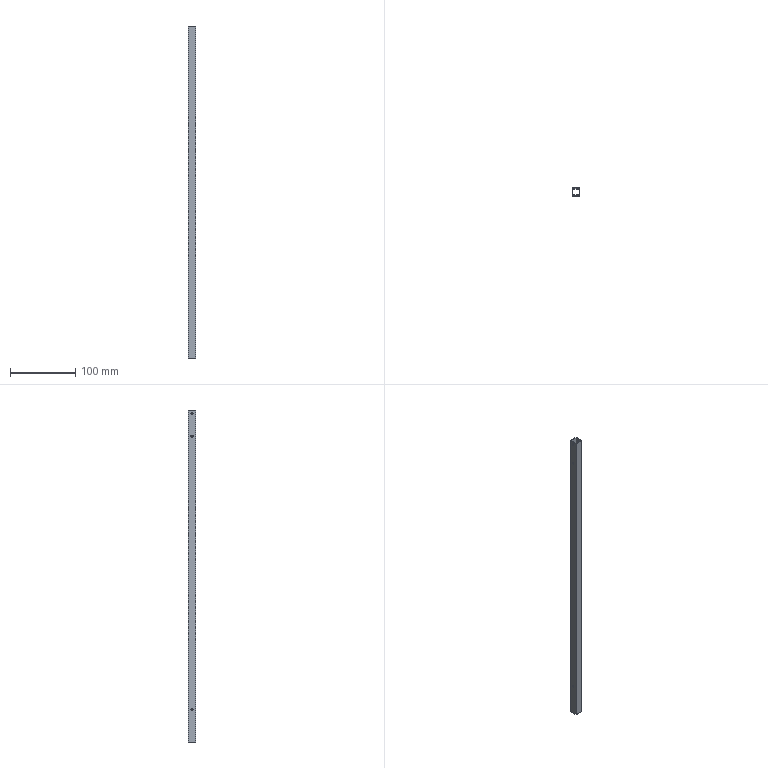Part | SolidWorks | features ICE 2, Extrusion 1 | 1 solid | 22 faces | box 12 x 12 x 508 mm | volume 22307 mm3 | cylinder 12 | plane 10 | commonest cylinder face diameters 3.1 x12
STEP:
#1=CARTESIAN_POINT('',(6.,0.,48.45));
#2=VERTEX_POINT('',#1);
#3=CARTESIAN_POINT('',(6.,0.,51.55));
#4=VERTEX_POINT('',#3);
#5=CARTESIAN_POINT('',(6.,0.,50.));
#6=DIRECTION('',(-1.,0.,0.));
#7=DIRECTION('',(0.,0.,1.));
#8=AXIS2_PLACEMENT_3D('',#5,#6,#7);
#9=CIRCLE('',#8,1.55);
#10=EDGE_CURVE('',#2,#4,#9,.T.);
#11=ORIENTED_EDGE('',*,*,#10,.F.);
#12=CARTESIAN_POINT('',(5.,0.,48.45));
#13=VERTEX_POINT('',#12);
#14=CARTESIAN_POINT('',(6.,0.,48.45));
#15=DIRECTION('',(-1.,0.,0.));
#16=VECTOR('',#15,1000.);
#17=LINE('',#14,#16);
#18=EDGE_CURVE('',#2,#13,#17,.T.);
#19=ORIENTED_EDGE('',*,*,#18,.T.);
#20=CARTESIAN_POINT('',(5.,0.,51.55));
#21=VERTEX_POINT('',#20);
#22=CARTESIAN_POINT('',(5.,0.,50.));
#23=DIRECTION('',(-1.,0.,0.));
#24=DIRECTION('',(0.,-1.,0.));
#25=AXIS2_PLACEMENT_3D('',#22,#23,#24);
#26=CIRCLE('',#25,1.55);
#27=EDGE_CURVE('',#13,#21,#26,.T.);
#28=ORIENTED_EDGE('',*,*,#27,.T.);
#29=CARTESIAN_POINT('',(6.,0.,51.55));
#30=DIRECTION('',(-1.,0.,0.));
#31=VECTOR('',#30,1000.);
#32=LINE('',#29,#31);
#33=EDGE_CURVE('',#4,#21,#32,.T.);
#34=ORIENTED_EDGE('',*,*,#33,.F.);
#35=EDGE_LOOP('',(#11,#19,#28,#34));
#36=FACE_OUTER_BOUND('',#35,.T.);
#37=CARTESIAN_POINT('',(6.,0.,50.));
#38=DIRECTION('',(-1.,0.,0.));
#39=DIRECTION('',(0.,0.,1.));
#40=AXIS2_PLACEMENT_3D('',#37,#38,#39);
#41=CYLINDRICAL_SURFACE('',#40,1.55);
#42=ADVANCED_FACE('',(#36),#41,.F.);
#43=CARTESIAN_POINT('',(6.,0.,466.583));
#44=VERTEX_POINT('',#43);
#45=CARTESIAN_POINT('',(6.,0.,469.683));
#46=VERTEX_POINT('',#45);
#47=CARTESIAN_POINT('',(6.,0.,468.133));
#48=DIRECTION('',(-1.,0.,0.));
#49=DIRECTION('',(0.,0.,1.));
#50=AXIS2_PLACEMENT_3D('',#47,#48,#49);
#51=CIRCLE('',#50,1.55);
#52=EDGE_CURVE('',#44,#46,#51,.T.);
#53=ORIENTED_EDGE('',*,*,#52,.F.);
#54=CARTESIAN_POINT('',(5.,0.,466.583));
#55=VERTEX_POINT('',#54);
#56=CARTESIAN_POINT('',(6.,0.,466.583));
#57=DIRECTION('',(-1.,0.,0.));
#58=VECTOR('',#57,1000.);
#59=LINE('',#56,#58);
#60=EDGE_CURVE('',#44,#55,#59,.T.);
#61=ORIENTED_EDGE('',*,*,#60,.T.);
#62=CARTESIAN_POINT('',(5.,0.,469.683));
#63=VERTEX_POINT('',#62);
#64=CARTESIAN_POINT('',(5.,0.,468.133));
#65=DIRECTION('',(-1.,0.,0.));
#66=DIRECTION('',(0.,-1.,0.));
#67=AXIS2_PLACEMENT_3D('',#64,#65,#66);
#68=CIRCLE('',#67,1.55);
#69=EDGE_CURVE('',#55,#63,#68,.T.);
#70=ORIENTED_EDGE('',*,*,#69,.T.);
#71=CARTESIAN_POINT('',(6.,0.,469.683));
#72=DIRECTION('',(-1.,0.,0.));
#73=VECTOR('',#72,1000.);
#74=LINE('',#71,#73);
#75=EDGE_CURVE('',#46,#63,#74,.T.);
#76=ORIENTED_EDGE('',*,*,#75,.F.);
#77=EDGE_LOOP('',(#53,#61,#70,#76));
#78=FACE_OUTER_BOUND('',#77,.T.);
#79=CARTESIAN_POINT('',(6.,0.,468.133));
#80=DIRECTION('',(-1.,0.,0.));
#81=DIRECTION('',(0.,0.,1.));
#82=AXIS2_PLACEMENT_3D('',#79,#80,#81);
#83=CYLINDRICAL_SURFACE('',#82,1.55);
#84=ADVANCED_FACE('',(#78),#83,.F.);
#85=CARTESIAN_POINT('',(6.,0.,501.583));
#86=VERTEX_POINT('',#85);
#87=CARTESIAN_POINT('',(6.,0.,504.683));
#88=VERTEX_POINT('',#87);
#89=CARTESIAN_POINT('',(6.,0.,503.133));
#90=DIRECTION('',(-1.,0.,0.));
#91=DIRECTION('',(0.,0.,1.));
#92=AXIS2_PLACEMENT_3D('',#89,#90,#91);
#93=CIRCLE('',#92,1.55);
#94=EDGE_CURVE('',#86,#88,#93,.T.);
#95=ORIENTED_EDGE('',*,*,#94,.F.);
#96=CARTESIAN_POINT('',(5.,0.,501.583));
#97=VERTEX_POINT('',#96);
#98=CARTESIAN_POINT('',(6.,0.,501.583));
#99=DIRECTION('',(-1.,0.,0.));
#100=VECTOR('',#99,1000.);
#101=LINE('',#98,#100);
#102=EDGE_CURVE('',#86,#97,#101,.T.);
#103=ORIENTED_EDGE('',*,*,#102,.T.);
#104=CARTESIAN_POINT('',(5.,0.,504.683));
#105=VERTEX_POINT('',#104);
#106=CARTESIAN_POINT('',(5.,0.,503.133));
#107=DIRECTION('',(-1.,0.,0.));
#108=DIRECTION('',(0.,-1.,0.));
#109=AXIS2_PLACEMENT_3D('',#106,#107,#108);
#110=CIRCLE('',#109,1.55);
#111=EDGE_CURVE('',#97,#105,#110,.T.);
#112=ORIENTED_EDGE('',*,*,#111,.T.);
#113=CARTESIAN_POINT('',(6.,0.,504.683));
#114=DIRECTION('',(-1.,0.,0.));
#115=VECTOR('',#114,1000.);
#116=LINE('',#113,#115);
#117=EDGE_CURVE('',#88,#105,#116,.T.);
#118=ORIENTED_EDGE('',*,*,#117,.F.);
#119=EDGE_LOOP('',(#95,#103,#112,#118));
#120=FACE_OUTER_BOUND('',#119,.T.);
#121=CARTESIAN_POINT('',(6.,0.,503.133));
#122=DIRECTION('',(-1.,0.,0.));
#123=DIRECTION('',(0.,0.,1.));
#124=AXIS2_PLACEMENT_3D('',#121,#122,#123);
#125=CYLINDRICAL_SURFACE('',#124,1.55);
#126=ADVANCED_FACE('',(#120),#125,.F.);
#127=CARTESIAN_POINT('',(-5.,0.,51.55));
#128=VERTEX_POINT('',#127);
#129=CARTESIAN_POINT('',(-5.,0.,48.45));
#130=VERTEX_POINT('',#129);
#131=CARTESIAN_POINT('',(-5.,0.,50.));
#132=DIRECTION('',(1.,0.,0.));
#133=DIRECTION('',(0.,0.,-1.));
#134=AXIS2_PLACEMENT_3D('',#131,#132,#133);
#135=CIRCLE('',#134,1.55);
#136=EDGE_CURVE('',#128,#130,#135,.T.);
#137=ORIENTED_EDGE('',*,*,#136,.T.);
#138=CARTESIAN_POINT('',(-6.,0.,48.45));
#139=VERTEX_POINT('',#138);
#140=CARTESIAN_POINT('',(6.,0.,48.45));
#141=DIRECTION('',(-1.,0.,0.));
#142=VECTOR('',#141,1000.);
#143=LINE('',#140,#142);
#144=EDGE_CURVE('',#130,#139,#143,.T.);
#145=ORIENTED_EDGE('',*,*,#144,.T.);
#146=CARTESIAN_POINT('',(-6.,0.,51.55));
#147=VERTEX_POINT('',#146);
#148=CARTESIAN_POINT('',(-6.,0.,50.));
#149=DIRECTION('',(1.,0.,0.));
#150=DIRECTION('',(0.,0.,-1.));
#151=AXIS2_PLACEMENT_3D('',#148,#149,#150);
#152=CIRCLE('',#151,1.55);
#153=EDGE_CURVE('',#147,#139,#152,.T.);
#154=ORIENTED_EDGE('',*,*,#153,.F.);
#155=CARTESIAN_POINT('',(6.,0.,51.55));
#156=DIRECTION('',(-1.,0.,0.));
#157=VECTOR('',#156,1000.);
#158=LINE('',#155,#157);
#159=EDGE_CURVE('',#128,#147,#158,.T.);
#160=ORIENTED_EDGE('',*,*,#159,.F.);
#161=EDGE_LOOP('',(#137,#145,#154,#160));
#162=FACE_OUTER_BOUND('',#161,.T.);
#163=CARTESIAN_POINT('',(6.,0.,50.));
#164=DIRECTION('',(-1.,0.,0.));
#165=DIRECTION('',(0.,0.,1.));
#166=AXIS2_PLACEMENT_3D('',#163,#164,#165);
#167=CYLINDRICAL_SURFACE('',#166,1.55);
#168=ADVANCED_FACE('',(#162),#167,.F.);
#169=CARTESIAN_POINT('',(-5.,0.,469.683));
#170=VERTEX_POINT('',#169);
#171=CARTESIAN_POINT('',(-5.,0.,466.583));
#172=VERTEX_POINT('',#171);
#173=CARTESIAN_POINT('',(-5.,0.,468.133));
#174=DIRECTION('',(1.,0.,0.));
#175=DIRECTION('',(0.,0.,-1.));
#176=AXIS2_PLACEMENT_3D('',#173,#174,#175);
#177=CIRCLE('',#176,1.55);
#178=EDGE_CURVE('',#170,#172,#177,.T.);
#179=ORIENTED_EDGE('',*,*,#178,.T.);
#180=CARTESIAN_POINT('',(-6.,0.,466.583));
#181=VERTEX_POINT('',#180);
#182=CARTESIAN_POINT('',(6.,0.,466.583));
#183=DIRECTION('',(-1.,0.,0.));
#184=VECTOR('',#183,1000.);
#185=LINE('',#182,#184);
#186=EDGE_CURVE('',#172,#181,#185,.T.);
#187=ORIENTED_EDGE('',*,*,#186,.T.);
#188=CARTESIAN_POINT('',(-6.,0.,469.683));
#189=VERTEX_POINT('',#188);
#190=CARTESIAN_POINT('',(-6.,0.,468.133));
#191=DIRECTION('',(1.,0.,0.));
#192=DIRECTION('',(0.,0.,-1.));
#193=AXIS2_PLACEMENT_3D('',#190,#191,#192);
#194=CIRCLE('',#193,1.55);
#195=EDGE_CURVE('',#189,#181,#194,.T.);
#196=ORIENTED_EDGE('',*,*,#195,.F.);
#197=CARTESIAN_POINT('',(6.,0.,469.683));
#198=DIRECTION('',(-1.,0.,0.));
#199=VECTOR('',#198,1000.);
#200=LINE('',#197,#199);
#201=EDGE_CURVE('',#170,#189,#200,.T.);
#202=ORIENTED_EDGE('',*,*,#201,.F.);
#203=EDGE_LOOP('',(#179,#187,#196,#202));
#204=FACE_OUTER_BOUND('',#203,.T.);
#205=CARTESIAN_POINT('',(6.,0.,468.133));
#206=DIRECTION('',(-1.,0.,0.));
#207=DIRECTION('',(0.,0.,1.));
#208=AXIS2_PLACEMENT_3D('',#205,#206,#207);
#209=CYLINDRICAL_SURFACE('',#208,1.55);
#210=ADVANCED_FACE('',(#204),#209,.F.);
#211=CARTESIAN_POINT('',(-5.,0.,504.683));
#212=VERTEX_POINT('',#211);
#213=CARTESIAN_POINT('',(-5.,0.,501.583));
#214=VERTEX_POINT('',#213);
#215=CARTESIAN_POINT('',(-5.,0.,503.133));
#216=DIRECTION('',(1.,0.,0.));
#217=DIRECTION('',(0.,0.,-1.));
#218=AXIS2_PLACEMENT_3D('',#215,#216,#217);
#219=CIRCLE('',#218,1.55);
#220=EDGE_CURVE('',#212,#214,#219,.T.);
#221=ORIENTED_EDGE('',*,*,#220,.T.);
#222=CARTESIAN_POINT('',(-6.,0.,501.583));
#223=VERTEX_POINT('',#222);
#224=CARTESIAN_POINT('',(6.,0.,501.583));
#225=DIRECTION('',(-1.,0.,0.));
#226=VECTOR('',#225,1000.);
#227=LINE('',#224,#226);
#228=EDGE_CURVE('',#214,#223,#227,.T.);
#229=ORIENTED_EDGE('',*,*,#228,.T.);
#230=CARTESIAN_POINT('',(-6.,0.,504.683));
#231=VERTEX_POINT('',#230);
#232=CARTESIAN_POINT('',(-6.,0.,503.133));
#233=DIRECTION('',(1.,0.,0.));
#234=DIRECTION('',(0.,0.,-1.));
#235=AXIS2_PLACEMENT_3D('',#232,#233,#234);
#236=CIRCLE('',#235,1.55);
#237=EDGE_CURVE('',#231,#223,#236,.T.);
#238=ORIENTED_EDGE('',*,*,#237,.F.);
#239=CARTESIAN_POINT('',(6.,0.,504.683));
#240=DIRECTION('',(-1.,0.,0.));
#241=VECTOR('',#240,1000.);
#242=LINE('',#239,#241);
#243=EDGE_CURVE('',#212,#231,#242,.T.);
#244=ORIENTED_EDGE('',*,*,#243,.F.);
#245=EDGE_LOOP('',(#221,#229,#238,#244));
#246=FACE_OUTER_BOUND('',#245,.T.);
#247=CARTESIAN_POINT('',(6.,0.,503.133));
#248=DIRECTION('',(-1.,0.,0.));
#249=DIRECTION('',(0.,0.,1.));
#250=AXIS2_PLACEMENT_3D('',#247,#248,#249);
#251=CYLINDRICAL_SURFACE('',#250,1.55);
#252=ADVANCED_FACE('',(#246),#251,.F.);
#253=CARTESIAN_POINT('',(6.,0.,503.133));
#254=DIRECTION('',(-1.,0.,0.));
#255=DIRECTION('',(0.,0.,1.));
#256=AXIS2_PLACEMENT_3D('',#253,#254,#255);
#257=CIRCLE('',#256,1.55);
#258=EDGE_CURVE('',#88,#86,#257,.T.);
#259=ORIENTED_EDGE('',*,*,#258,.T.);
#260=ORIENTED_EDGE('',*,*,#94,.T.);
#261=EDGE_LOOP('',(#259,#260));
#262=FACE_BOUND('',#261,.T.);
#263=CARTESIAN_POINT('',(6.,0.,468.133));
#264=DIRECTION('',(-1.,0.,0.));
#265=DIRECTION('',(0.,0.,1.));
#266=AXIS2_PLACEMENT_3D('',#263,#264,#265);
#267=CIRCLE('',#266,1.55);
#268=EDGE_CURVE('',#46,#44,#267,.T.);
#269=ORIENTED_EDGE('',*,*,#268,.T.);
#270=ORIENTED_EDGE('',*,*,#52,.T.);
#271=EDGE_LOOP('',(#269,#270));
#272=FACE_BOUND('',#271,.T.);
#273=CARTESIAN_POINT('',(6.,0.,50.));
#274=DIRECTION('',(-1.,0.,0.));
#275=DIRECTION('',(0.,0.,1.));
#276=AXIS2_PLACEMENT_3D('',#273,#274,#275);
#277=CIRCLE('',#276,1.55);
#278=EDGE_CURVE('',#4,#2,#277,.T.);
#279=ORIENTED_EDGE('',*,*,#278,.T.);
#280=ORIENTED_EDGE('',*,*,#10,.T.);
#281=EDGE_LOOP('',(#279,#280));
#282=FACE_BOUND('',#281,.T.);
#283=CARTESIAN_POINT('',(6.,-6.,508.));
#284=VERTEX_POINT('',#283);
#285=CARTESIAN_POINT('',(6.,6.,508.));
#286=VERTEX_POINT('',#285);
#287=CARTESIAN_POINT('',(6.,-6.,508.));
#288=DIRECTION('',(0.,1.,0.));
#289=VECTOR('',#288,1000.);
#290=LINE('',#287,#289);
#291=EDGE_CURVE('',#284,#286,#290,.T.);
#292=ORIENTED_EDGE('',*,*,#291,.F.);
#293=CARTESIAN_POINT('',(6.,-6.,0.));
#294=VERTEX_POINT('',#293);
#295=CARTESIAN_POINT('',(6.,-6.,516.));
#296=DIRECTION('',(0.,0.,-1.));
#297=VECTOR('',#296,1000.);
#298=LINE('',#295,#297);
#299=EDGE_CURVE('',#284,#294,#298,.T.);
#300=ORIENTED_EDGE('',*,*,#299,.T.);
#301=CARTESIAN_POINT('',(6.,6.,0.));
#302=VERTEX_POINT('',#301);
#303=CARTESIAN_POINT('',(6.,-6.,0.));
#304=DIRECTION('',(0.,1.,0.));
#305=VECTOR('',#304,1000.);
#306=LINE('',#303,#305);
#307=EDGE_CURVE('',#294,#302,#306,.T.);
#308=ORIENTED_EDGE('',*,*,#307,.T.);
#309=CARTESIAN_POINT('',(6.,6.,516.));
#310=DIRECTION('',(0.,0.,-1.));
#311=VECTOR('',#310,1000.);
#312=LINE('',#309,#311);
#313=EDGE_CURVE('',#286,#302,#312,.T.);
#314=ORIENTED_EDGE('',*,*,#313,.F.);
#315=EDGE_LOOP('',(#292,#300,#308,#314));
#316=FACE_OUTER_BOUND('',#315,.T.);
#317=CARTESIAN_POINT('',(6.,-6.,516.));
#318=DIRECTION('',(-1.,0.,0.));
#319=DIRECTION('',(0.,0.,1.));
#320=AXIS2_PLACEMENT_3D('',#317,#318,#319);
#321=PLANE('',#320);
#322=ADVANCED_FACE('',(#262,#272,#282,#316),#321,.F.);
#323=CARTESIAN_POINT('',(-6.,6.,508.));
#324=VERTEX_POINT('',#323);
#325=CARTESIAN_POINT('',(6.,6.,508.));
#326=DIRECTION('',(-1.,0.,0.));
#327=VECTOR('',#326,1000.);
#328=LINE('',#325,#327);
#329=EDGE_CURVE('',#286,#324,#328,.T.);
#330=ORIENTED_EDGE('',*,*,#329,.F.);
#331=ORIENTED_EDGE('',*,*,#313,.T.);
#332=CARTESIAN_POINT('',(-6.,6.,0.));
#333=VERTEX_POINT('',#332);
#334=CARTESIAN_POINT('',(-6.,6.,0.));
#335=DIRECTION('',(-1.,0.,0.));
#336=VECTOR('',#335,1000.);
#337=LINE('',#334,#336);
#338=EDGE_CURVE('',#302,#333,#337,.T.);
#339=ORIENTED_EDGE('',*,*,#338,.T.);
#340=CARTESIAN_POINT('',(-6.,6.,516.));
#341=DIRECTION('',(0.,0.,-1.));
#342=VECTOR('',#341,1000.);
#343=LINE('',#340,#342);
#344=EDGE_CURVE('',#324,#333,#343,.T.);
#345=ORIENTED_EDGE('',*,*,#344,.F.);
#346=EDGE_LOOP('',(#330,#331,#339,#345));
#347=FACE_OUTER_BOUND('',#346,.T.);
#348=CARTESIAN_POINT('',(-6.,6.,516.));
#349=DIRECTION('',(0.,-1.,0.));
#350=DIRECTION('',(0.,0.,-1.));
#351=AXIS2_PLACEMENT_3D('',#348,#349,#350);
#352=PLANE('',#351);
#353=ADVANCED_FACE('',(#347),#352,.F.);
#354=ORIENTED_EDGE('',*,*,#237,.T.);
#355=CARTESIAN_POINT('',(-6.,0.,503.133));
#356=DIRECTION('',(1.,0.,0.));
#357=DIRECTION('',(0.,0.,-1.));
#358=AXIS2_PLACEMENT_3D('',#355,#356,#357);
#359=CIRCLE('',#358,1.55);
#360=EDGE_CURVE('',#223,#231,#359,.T.);
#361=ORIENTED_EDGE('',*,*,#360,.T.);
#362=EDGE_LOOP('',(#354,#361));
#363=FACE_BOUND('',#362,.T.);
#364=ORIENTED_EDGE('',*,*,#195,.T.);
#365=CARTESIAN_POINT('',(-6.,0.,468.133));
#366=DIRECTION('',(1.,0.,0.));
#367=DIRECTION('',(0.,0.,-1.));
#368=AXIS2_PLACEMENT_3D('',#365,#366,#367);
#369=CIRCLE('',#368,1.55);
#370=EDGE_CURVE('',#181,#189,#369,.T.);
#371=ORIENTED_EDGE('',*,*,#370,.T.);
#372=EDGE_LOOP('',(#364,#371));
#373=FACE_BOUND('',#372,.T.);
#374=ORIENTED_EDGE('',*,*,#153,.T.);
#375=CARTESIAN_POINT('',(-6.,0.,50.));
#376=DIRECTION('',(1.,0.,0.));
#377=DIRECTION('',(0.,0.,-1.));
#378=AXIS2_PLACEMENT_3D('',#375,#376,#377);
#379=CIRCLE('',#378,1.55);
#380=EDGE_CURVE('',#139,#147,#379,.T.);
#381=ORIENTED_EDGE('',*,*,#380,.T.);
#382=EDGE_LOOP('',(#374,#381));
#383=FACE_BOUND('',#382,.T.);
#384=CARTESIAN_POINT('',(-6.,-6.,508.));
#385=VERTEX_POINT('',#384);
#386=CARTESIAN_POINT('',(-6.,6.,508.));
#387=DIRECTION('',(0.,-1.,0.));
#388=VECTOR('',#387,1000.);
#389=LINE('',#386,#388);
#390=EDGE_CURVE('',#324,#385,#389,.T.);
#391=ORIENTED_EDGE('',*,*,#390,.F.);
#392=ORIENTED_EDGE('',*,*,#344,.T.);
#393=CARTESIAN_POINT('',(-6.,-6.,0.));
#394=VERTEX_POINT('',#393);
#395=CARTESIAN_POINT('',(-6.,-6.,0.));
#396=DIRECTION('',(0.,-1.,0.));
#397=VECTOR('',#396,1000.);
#398=LINE('',#395,#397);
#399=EDGE_CURVE('',#333,#394,#398,.T.);
#400=ORIENTED_EDGE('',*,*,#399,.T.);
#401=CARTESIAN_POINT('',(-6.,-6.,516.));
#402=DIRECTION('',(0.,0.,-1.));
#403=VECTOR('',#402,1000.);
#404=LINE('',#401,#403);
#405=EDGE_CURVE('',#385,#394,#404,.T.);
#406=ORIENTED_EDGE('',*,*,#405,.F.);
#407=EDGE_LOOP('',(#391,#392,#400,#406));
#408=FACE_OUTER_BOUND('',#407,.T.);
#409=CARTESIAN_POINT('',(-6.,-6.,516.));
#410=DIRECTION('',(1.,0.,0.));
#411=DIRECTION('',(0.,0.,-1.));
#412=AXIS2_PLACEMENT_3D('',#409,#410,#411);
#413=PLANE('',#412);
#414=ADVANCED_FACE('',(#363,#373,#383,#408),#413,.F.);
#415=CARTESIAN_POINT('',(-6.,-6.,508.));
#416=DIRECTION('',(1.,0.,0.));
#417=VECTOR('',#416,1000.);
#418=LINE('',#415,#417);
#419=EDGE_CURVE('',#385,#284,#418,.T.);
#420=ORIENTED_EDGE('',*,*,#419,.F.);
#421=ORIENTED_EDGE('',*,*,#405,.T.);
#422=CARTESIAN_POINT('',(-6.,-6.,0.));
#423=DIRECTION('',(1.,0.,0.));
#424=VECTOR('',#423,1000.);
#425=LINE('',#422,#424);
#426=EDGE_CURVE('',#394,#294,#425,.T.);
#427=ORIENTED_EDGE('',*,*,#426,.T.);
#428=ORIENTED_EDGE('',*,*,#299,.F.);
#429=EDGE_LOOP('',(#420,#421,#427,#428));
#430=FACE_OUTER_BOUND('',#429,.T.);
#431=CARTESIAN_POINT('',(-6.,-6.,516.));
#432=DIRECTION('',(0.,1.,0.));
#433=DIRECTION('',(0.,0.,1.));
#434=AXIS2_PLACEMENT_3D('',#431,#432,#433);
#435=PLANE('',#434);
#436=ADVANCED_FACE('',(#430),#435,.F.);
#437=CARTESIAN_POINT('',(-5.,-5.,508.));
#438=VERTEX_POINT('',#437);
#439=CARTESIAN_POINT('',(-5.,-5.,0.));
#440=VERTEX_POINT('',#439);
#441=CARTESIAN_POINT('',(-5.,-5.,516.));
#442=DIRECTION('',(0.,0.,-1.));
#443=VECTOR('',#442,1000.);
#444=LINE('',#441,#443);
#445=EDGE_CURVE('',#438,#440,#444,.T.);
#446=ORIENTED_EDGE('',*,*,#445,.F.);
#447=CARTESIAN_POINT('',(5.,-5.,508.));
#448=VERTEX_POINT('',#447);
#449=CARTESIAN_POINT('',(-5.,-5.,508.));
#450=DIRECTION('',(1.,0.,0.));
#451=VECTOR('',#450,1000.);
#452=LINE('',#449,#451);
#453=EDGE_CURVE('',#438,#448,#452,.T.);
#454=ORIENTED_EDGE('',*,*,#453,.T.);
#455=CARTESIAN_POINT('',(5.,-5.,0.));
#456=VERTEX_POINT('',#455);
#457=CARTESIAN_POINT('',(5.,-5.,516.));
#458=DIRECTION('',(0.,0.,-1.));
#459=VECTOR('',#458,1000.);
#460=LINE('',#457,#459);
#461=EDGE_CURVE('',#448,#456,#460,.T.);
#462=ORIENTED_EDGE('',*,*,#461,.T.);
#463=CARTESIAN_POINT('',(-5.,-5.,0.));
#464=DIRECTION('',(1.,0.,0.));
#465=VECTOR('',#464,1000.);
#466=LINE('',#463,#465);
#467=EDGE_CURVE('',#440,#456,#466,.T.);
#468=ORIENTED_EDGE('',*,*,#467,.F.);
#469=EDGE_LOOP('',(#446,#454,#462,#468));
#470=FACE_OUTER_BOUND('',#469,.T.);
#471=CARTESIAN_POINT('',(-5.,-5.,516.));
#472=DIRECTION('',(0.,1.,0.));
#473=DIRECTION('',(0.,0.,1.));
#474=AXIS2_PLACEMENT_3D('',#471,#472,#473);
#475=PLANE('',#474);
#476=ADVANCED_FACE('',(#470),#475,.T.);
#477=CARTESIAN_POINT('',(5.,0.,50.));
#478=DIRECTION('',(-1.,0.,0.));
#479=DIRECTION('',(0.,-1.,0.));
#480=AXIS2_PLACEMENT_3D('',#477,#478,#479);
#481=CIRCLE('',#480,1.55);
#482=EDGE_CURVE('',#21,#13,#481,.T.);
#483=ORIENTED_EDGE('',*,*,#482,.F.);
#484=ORIENTED_EDGE('',*,*,#27,.F.);
#485=EDGE_LOOP('',(#483,#484));
#486=FACE_BOUND('',#485,.T.);
#487=CARTESIAN_POINT('',(5.,0.,468.133));
#488=DIRECTION('',(-1.,0.,0.));
#489=DIRECTION('',(0.,-1.,0.));
#490=AXIS2_PLACEMENT_3D('',#487,#488,#489);
#491=CIRCLE('',#490,1.55);
#492=EDGE_CURVE('',#63,#55,#491,.T.);
#493=ORIENTED_EDGE('',*,*,#492,.F.);
#494=ORIENTED_EDGE('',*,*,#69,.F.);
#495=EDGE_LOOP('',(#493,#494));
#496=FACE_BOUND('',#495,.T.);
#497=CARTESIAN_POINT('',(5.,0.,503.133));
#498=DIRECTION('',(-1.,0.,0.));
#499=DIRECTION('',(0.,-1.,0.));
#500=AXIS2_PLACEMENT_3D('',#497,#498,#499);
#501=CIRCLE('',#500,1.55);
#502=EDGE_CURVE('',#105,#97,#501,.T.);
#503=ORIENTED_EDGE('',*,*,#502,.F.);
#504=ORIENTED_EDGE('',*,*,#111,.F.);
#505=EDGE_LOOP('',(#503,#504));
#506=FACE_BOUND('',#505,.T.);
#507=ORIENTED_EDGE('',*,*,#461,.F.);
#508=CARTESIAN_POINT('',(5.,5.,508.));
#509=VERTEX_POINT('',#508);
#510=CARTESIAN_POINT('',(5.,-5.,508.));
#511=DIRECTION('',(0.,1.,0.));
#512=VECTOR('',#511,1000.);
#513=LINE('',#510,#512);
#514=EDGE_CURVE('',#448,#509,#513,.T.);
#515=ORIENTED_EDGE('',*,*,#514,.T.);
#516=CARTESIAN_POINT('',(5.,5.,0.));
#517=VERTEX_POINT('',#516);
#518=CARTESIAN_POINT('',(5.,5.,516.));
#519=DIRECTION('',(0.,0.,-1.));
#520=VECTOR('',#519,1000.);
#521=LINE('',#518,#520);
#522=EDGE_CURVE('',#509,#517,#521,.T.);
#523=ORIENTED_EDGE('',*,*,#522,.T.);
#524=CARTESIAN_POINT('',(5.,-5.,0.));
#525=DIRECTION('',(0.,1.,0.));
#526=VECTOR('',#525,1000.);
#527=LINE('',#524,#526);
#528=EDGE_CURVE('',#456,#517,#527,.T.);
#529=ORIENTED_EDGE('',*,*,#528,.F.);
#530=EDGE_LOOP('',(#507,#515,#523,#529));
#531=FACE_OUTER_BOUND('',#530,.T.);
#532=CARTESIAN_POINT('',(5.,-5.,516.));
#533=DIRECTION('',(-1.,0.,0.));
#534=DIRECTION('',(0.,-1.,0.));
#535=AXIS2_PLACEMENT_3D('',#532,#533,#534);
#536=PLANE('',#535);
#537=ADVANCED_FACE('',(#486,#496,#506,#531),#536,.T.);
#538=ORIENTED_EDGE('',*,*,#522,.F.);
#539=CARTESIAN_POINT('',(-5.,5.,508.));
#540=VERTEX_POINT('',#539);
#541=CARTESIAN_POINT('',(5.,5.,508.));
#542=DIRECTION('',(-1.,0.,0.));
#543=VECTOR('',#542,1000.);
#544=LINE('',#541,#543);
#545=EDGE_CURVE('',#509,#540,#544,.T.);
#546=ORIENTED_EDGE('',*,*,#545,.T.);
#547=CARTESIAN_POINT('',(-5.,5.,0.));
#548=VERTEX_POINT('',#547);
#549=CARTESIAN_POINT('',(-5.,5.,516.));
#550=DIRECTION('',(0.,0.,-1.));
#551=VECTOR('',#550,1000.);
#552=LINE('',#549,#551);
#553=EDGE_CURVE('',#540,#548,#552,.T.);
#554=ORIENTED_EDGE('',*,*,#553,.T.);
#555=CARTESIAN_POINT('',(-5.,5.,0.));
#556=DIRECTION('',(-1.,0.,0.));
#557=VECTOR('',#556,1000.);
#558=LINE('',#555,#557);
#559=EDGE_CURVE('',#517,#548,#558,.T.);
#560=ORIENTED_EDGE('',*,*,#559,.F.);
#561=EDGE_LOOP('',(#538,#546,#554,#560));
#562=FACE_OUTER_BOUND('',#561,.T.);
#563=CARTESIAN_POINT('',(-5.,5.,516.));
#564=DIRECTION('',(0.,-1.,0.));
#565=DIRECTION('',(0.,0.,-1.));
#566=AXIS2_PLACEMENT_3D('',#563,#564,#565);
#567=PLANE('',#566);
#568=ADVANCED_FACE('',(#562),#567,.T.);
#569=ORIENTED_EDGE('',*,*,#136,.F.);
#570=CARTESIAN_POINT('',(-5.,0.,50.));
#571=DIRECTION('',(1.,0.,0.));
#572=DIRECTION('',(0.,0.,-1.));
#573=AXIS2_PLACEMENT_3D('',#570,#571,#572);
#574=CIRCLE('',#573,1.55);
#575=EDGE_CURVE('',#130,#128,#574,.T.);
#576=ORIENTED_EDGE('',*,*,#575,.F.);
#577=EDGE_LOOP('',(#569,#576));
#578=FACE_BOUND('',#577,.T.);
#579=ORIENTED_EDGE('',*,*,#178,.F.);
#580=CARTESIAN_POINT('',(-5.,0.,468.133));
#581=DIRECTION('',(1.,0.,0.));
#582=DIRECTION('',(0.,0.,-1.));
#583=AXIS2_PLACEMENT_3D('',#580,#581,#582);
#584=CIRCLE('',#583,1.55);
#585=EDGE_CURVE('',#172,#170,#584,.T.);
#586=ORIENTED_EDGE('',*,*,#585,.F.);
#587=EDGE_LOOP('',(#579,#586));
#588=FACE_BOUND('',#587,.T.);
#589=ORIENTED_EDGE('',*,*,#220,.F.);
#590=CARTESIAN_POINT('',(-5.,0.,503.133));
#591=DIRECTION('',(1.,0.,0.));
#592=DIRECTION('',(0.,0.,-1.));
#593=AXIS2_PLACEMENT_3D('',#590,#591,#592);
#594=CIRCLE('',#593,1.55);
#595=EDGE_CURVE('',#214,#212,#594,.T.);
#596=ORIENTED_EDGE('',*,*,#595,.F.);
#597=EDGE_LOOP('',(#589,#596));
#598=FACE_BOUND('',#597,.T.);
#599=ORIENTED_EDGE('',*,*,#553,.F.);
#600=CARTESIAN_POINT('',(-5.,5.,508.));
#601=DIRECTION('',(0.,-1.,0.));
#602=VECTOR('',#601,1000.);
#603=LINE('',#600,#602);
#604=EDGE_CURVE('',#540,#438,#603,.T.);
#605=ORIENTED_EDGE('',*,*,#604,.T.);
#606=ORIENTED_EDGE('',*,*,#445,.T.);
#607=CARTESIAN_POINT('',(-5.,-5.,0.));
#608=DIRECTION('',(0.,-1.,0.));
#609=VECTOR('',#608,1000.);
#610=LINE('',#607,#609);
#611=EDGE_CURVE('',#548,#440,#610,.T.);
#612=ORIENTED_EDGE('',*,*,#611,.F.);
#613=EDGE_LOOP('',(#599,#605,#606,#612));
#614=FACE_OUTER_BOUND('',#613,.T.);
#615=CARTESIAN_POINT('',(-5.,-5.,516.));
#616=DIRECTION('',(1.,0.,0.));
#617=DIRECTION('',(0.,0.,-1.));
#618=AXIS2_PLACEMENT_3D('',#615,#616,#617);
#619=PLANE('',#618);
#620=ADVANCED_FACE('',(#578,#588,#598,#614),#619,.T.);
#621=ORIENTED_EDGE('',*,*,#307,.F.);
#622=ORIENTED_EDGE('',*,*,#426,.F.);
#623=ORIENTED_EDGE('',*,*,#399,.F.);
#624=ORIENTED_EDGE('',*,*,#338,.F.);
#625=EDGE_LOOP('',(#621,#622,#623,#624));
#626=FACE_OUTER_BOUND('',#625,.T.);
#627=ORIENTED_EDGE('',*,*,#611,.T.);
#628=ORIENTED_EDGE('',*,*,#467,.T.);
#629=ORIENTED_EDGE('',*,*,#528,.T.);
#630=ORIENTED_EDGE('',*,*,#559,.T.);
#631=EDGE_LOOP('',(#627,#628,#629,#630));
#632=FACE_BOUND('',#631,.T.);
#633=CARTESIAN_POINT('',(0.,0.,0.));
#634=DIRECTION('',(0.,0.,-1.));
#635=DIRECTION('',(-1.,0.,0.));
#636=AXIS2_PLACEMENT_3D('',#633,#634,#635);
#637=PLANE('',#636);
#638=ADVANCED_FACE('',(#626,#632),#637,.T.);
#639=ORIENTED_EDGE('',*,*,#228,.F.);
#640=ORIENTED_EDGE('',*,*,#595,.T.);
#641=ORIENTED_EDGE('',*,*,#243,.T.);
#642=ORIENTED_EDGE('',*,*,#360,.F.);
#643=EDGE_LOOP('',(#639,#640,#641,#642));
#644=FACE_OUTER_BOUND('',#643,.T.);
#645=CARTESIAN_POINT('',(6.,0.,503.133));
#646=DIRECTION('',(-1.,0.,0.));
#647=DIRECTION('',(0.,0.,1.));
#648=AXIS2_PLACEMENT_3D('',#645,#646,#647);
#649=CYLINDRICAL_SURFACE('',#648,1.55);
#650=ADVANCED_FACE('',(#644),#649,.F.);
#651=ORIENTED_EDGE('',*,*,#186,.F.);
#652=ORIENTED_EDGE('',*,*,#585,.T.);
#653=ORIENTED_EDGE('',*,*,#201,.T.);
#654=ORIENTED_EDGE('',*,*,#370,.F.);
#655=EDGE_LOOP('',(#651,#652,#653,#654));
#656=FACE_OUTER_BOUND('',#655,.T.);
#657=CARTESIAN_POINT('',(6.,0.,468.133));
#658=DIRECTION('',(-1.,0.,0.));
#659=DIRECTION('',(0.,0.,1.));
#660=AXIS2_PLACEMENT_3D('',#657,#658,#659);
#661=CYLINDRICAL_SURFACE('',#660,1.55);
#662=ADVANCED_FACE('',(#656),#661,.F.);
#663=ORIENTED_EDGE('',*,*,#144,.F.);
#664=ORIENTED_EDGE('',*,*,#575,.T.);
#665=ORIENTED_EDGE('',*,*,#159,.T.);
#666=ORIENTED_EDGE('',*,*,#380,.F.);
#667=EDGE_LOOP('',(#663,#664,#665,#666));
#668=FACE_OUTER_BOUND('',#667,.T.);
#669=CARTESIAN_POINT('',(6.,0.,50.));
#670=DIRECTION('',(-1.,0.,0.));
#671=DIRECTION('',(0.,0.,1.));
#672=AXIS2_PLACEMENT_3D('',#669,#670,#671);
#673=CYLINDRICAL_SURFACE('',#672,1.55);
#674=ADVANCED_FACE('',(#668),#673,.F.);
#675=ORIENTED_EDGE('',*,*,#102,.F.);
#676=ORIENTED_EDGE('',*,*,#258,.F.);
#677=ORIENTED_EDGE('',*,*,#117,.T.);
#678=ORIENTED_EDGE('',*,*,#502,.T.);
#679=EDGE_LOOP('',(#675,#676,#677,#678));
#680=FACE_OUTER_BOUND('',#679,.T.);
#681=CARTESIAN_POINT('',(6.,0.,503.133));
#682=DIRECTION('',(-1.,0.,0.));
#683=DIRECTION('',(0.,0.,1.));
#684=AXIS2_PLACEMENT_3D('',#681,#682,#683);
#685=CYLINDRICAL_SURFACE('',#684,1.55);
#686=ADVANCED_FACE('',(#680),#685,.F.);
#687=ORIENTED_EDGE('',*,*,#60,.F.);
#688=ORIENTED_EDGE('',*,*,#268,.F.);
#689=ORIENTED_EDGE('',*,*,#75,.T.);
#690=ORIENTED_EDGE('',*,*,#492,.T.);
#691=EDGE_LOOP('',(#687,#688,#689,#690));
#692=FACE_OUTER_BOUND('',#691,.T.);
#693=CARTESIAN_POINT('',(6.,0.,468.133));
#694=DIRECTION('',(-1.,0.,0.));
#695=DIRECTION('',(0.,0.,1.));
#696=AXIS2_PLACEMENT_3D('',#693,#694,#695);
#697=CYLINDRICAL_SURFACE('',#696,1.55);
#698=ADVANCED_FACE('',(#692),#697,.F.);
#699=ORIENTED_EDGE('',*,*,#18,.F.);
#700=ORIENTED_EDGE('',*,*,#278,.F.);
#701=ORIENTED_EDGE('',*,*,#33,.T.);
#702=ORIENTED_EDGE('',*,*,#482,.T.);
#703=EDGE_LOOP('',(#699,#700,#701,#702));
#704=FACE_OUTER_BOUND('',#703,.T.);
#705=CARTESIAN_POINT('',(6.,0.,50.));
#706=DIRECTION('',(-1.,0.,0.));
#707=DIRECTION('',(0.,0.,1.));
#708=AXIS2_PLACEMENT_3D('',#705,#706,#707);
#709=CYLINDRICAL_SURFACE('',#708,1.55);
#710=ADVANCED_FACE('',(#704),#709,.F.);
#711=ORIENTED_EDGE('',*,*,#545,.F.);
#712=ORIENTED_EDGE('',*,*,#514,.F.);
#713=ORIENTED_EDGE('',*,*,#453,.F.);
#714=ORIENTED_EDGE('',*,*,#604,.F.);
#715=EDGE_LOOP('',(#711,#712,#713,#714));
#716=FACE_BOUND('',#715,.T.);
#717=ORIENTED_EDGE('',*,*,#419,.T.);
#718=ORIENTED_EDGE('',*,*,#291,.T.);
#719=ORIENTED_EDGE('',*,*,#329,.T.);
#720=ORIENTED_EDGE('',*,*,#390,.T.);
#721=EDGE_LOOP('',(#717,#718,#719,#720));
#722=FACE_OUTER_BOUND('',#721,.T.);
#723=CARTESIAN_POINT('',(0.,0.,508.));
#724=DIRECTION('',(0.,0.,1.));
#725=DIRECTION('',(1.,0.,0.));
#726=AXIS2_PLACEMENT_3D('',#723,#724,#725);
#727=PLANE('',#726);
#728=ADVANCED_FACE('',(#716,#722),#727,.T.);
#729=CLOSED_SHELL('',(#42,#84,#126,#168,#210,#252,#322,#353,#414,#436,#476,#537,#568,#620,#638,#650,#662,#674,#686,#698,#710,#728));
#730=MANIFOLD_SOLID_BREP('',#729);
#731=CARTESIAN_POINT('',(0.,0.,0.));
#732=DIRECTION('',(0.,0.,1.));
#733=DIRECTION('',(1.,0.,0.));
#734=AXIS2_PLACEMENT_3D('',#731,#732,#733);
#735=(LENGTH_UNIT()NAMED_UNIT(*)SI_UNIT(.MILLI.,.METRE.));
#736=UNCERTAINTY_MEASURE_WITH_UNIT(LENGTH_MEASURE(0.00001),#735,'','');
#737=(NAMED_UNIT(*)PLANE_ANGLE_UNIT()SI_UNIT($,.RADIAN.));
#738=(NAMED_UNIT(*)SI_UNIT($,.STERADIAN.)SOLID_ANGLE_UNIT());
#739=(GEOMETRIC_REPRESENTATION_CONTEXT(3)GLOBAL_UNCERTAINTY_ASSIGNED_CONTEXT((#736))GLOBAL_UNIT_ASSIGNED_CONTEXT((#735,#737,#738))REPRESENTATION_CONTEXT('',''));
#740=ADVANCED_BREP_SHAPE_REPRESENTATION('',(#730,#734),#739);